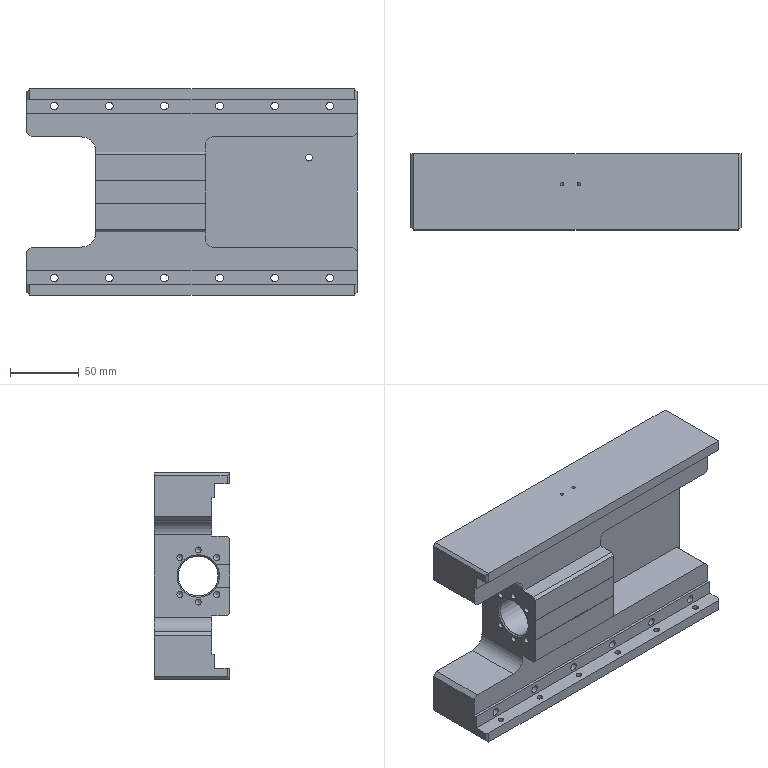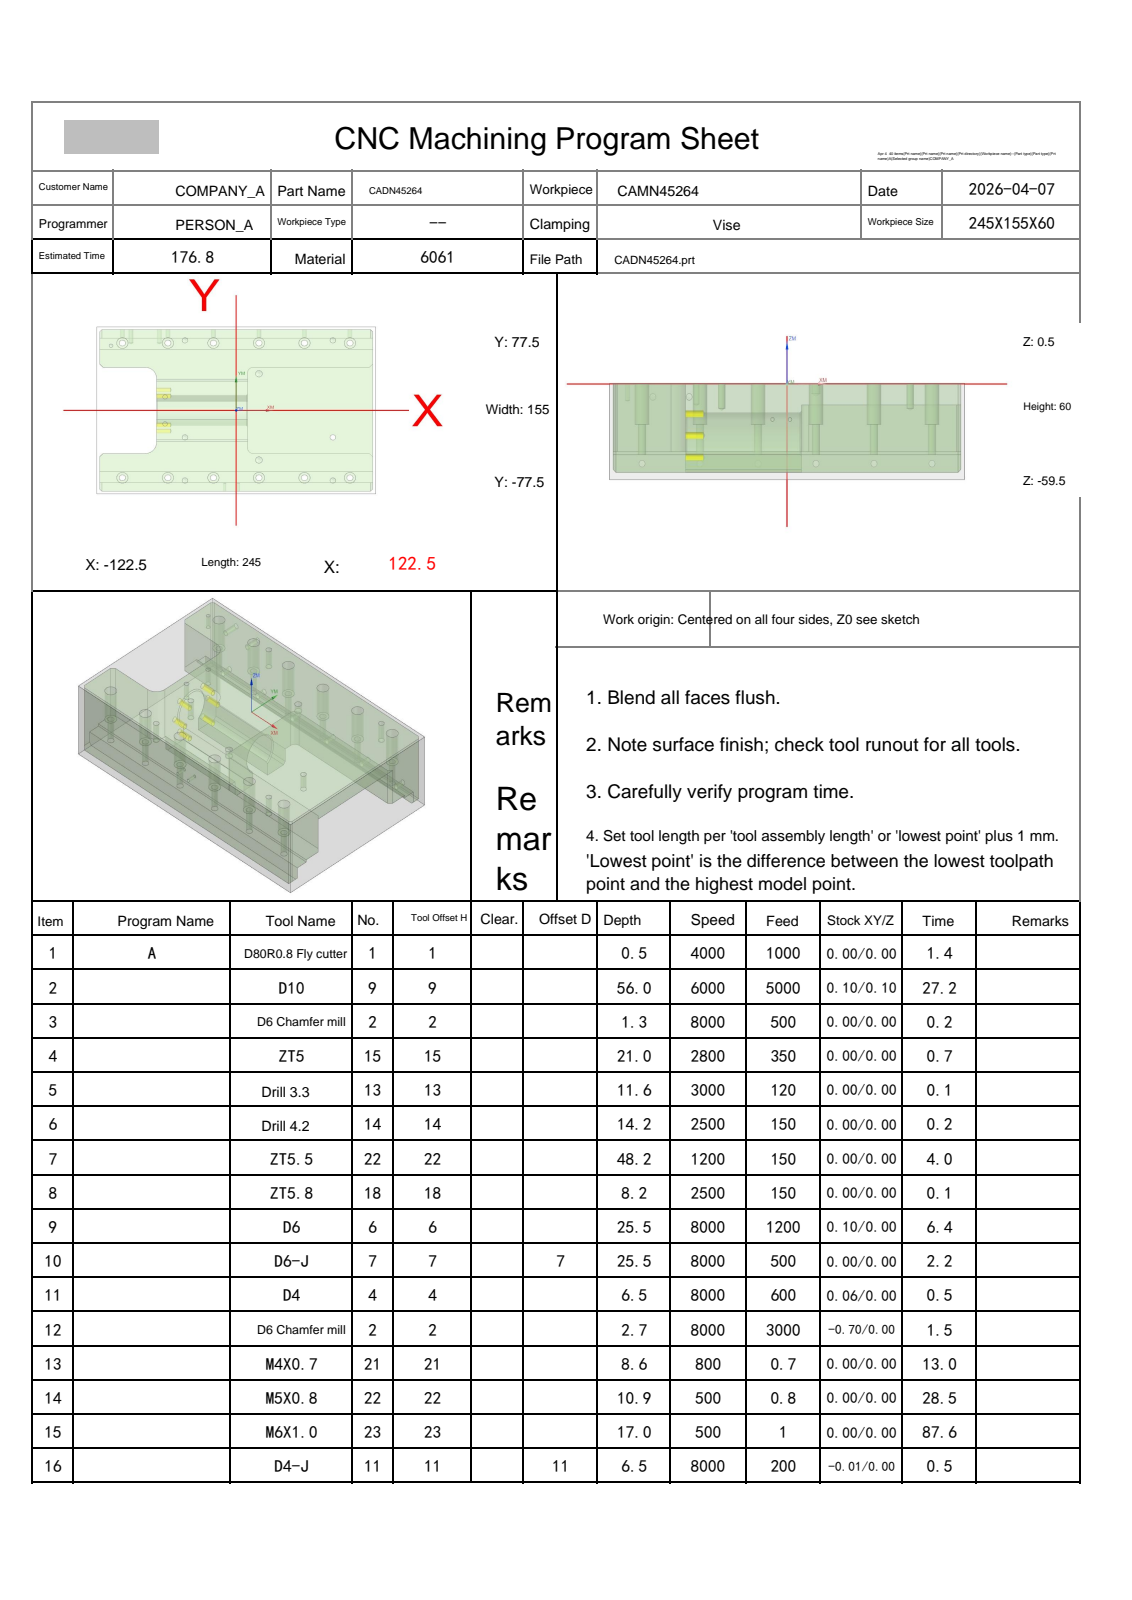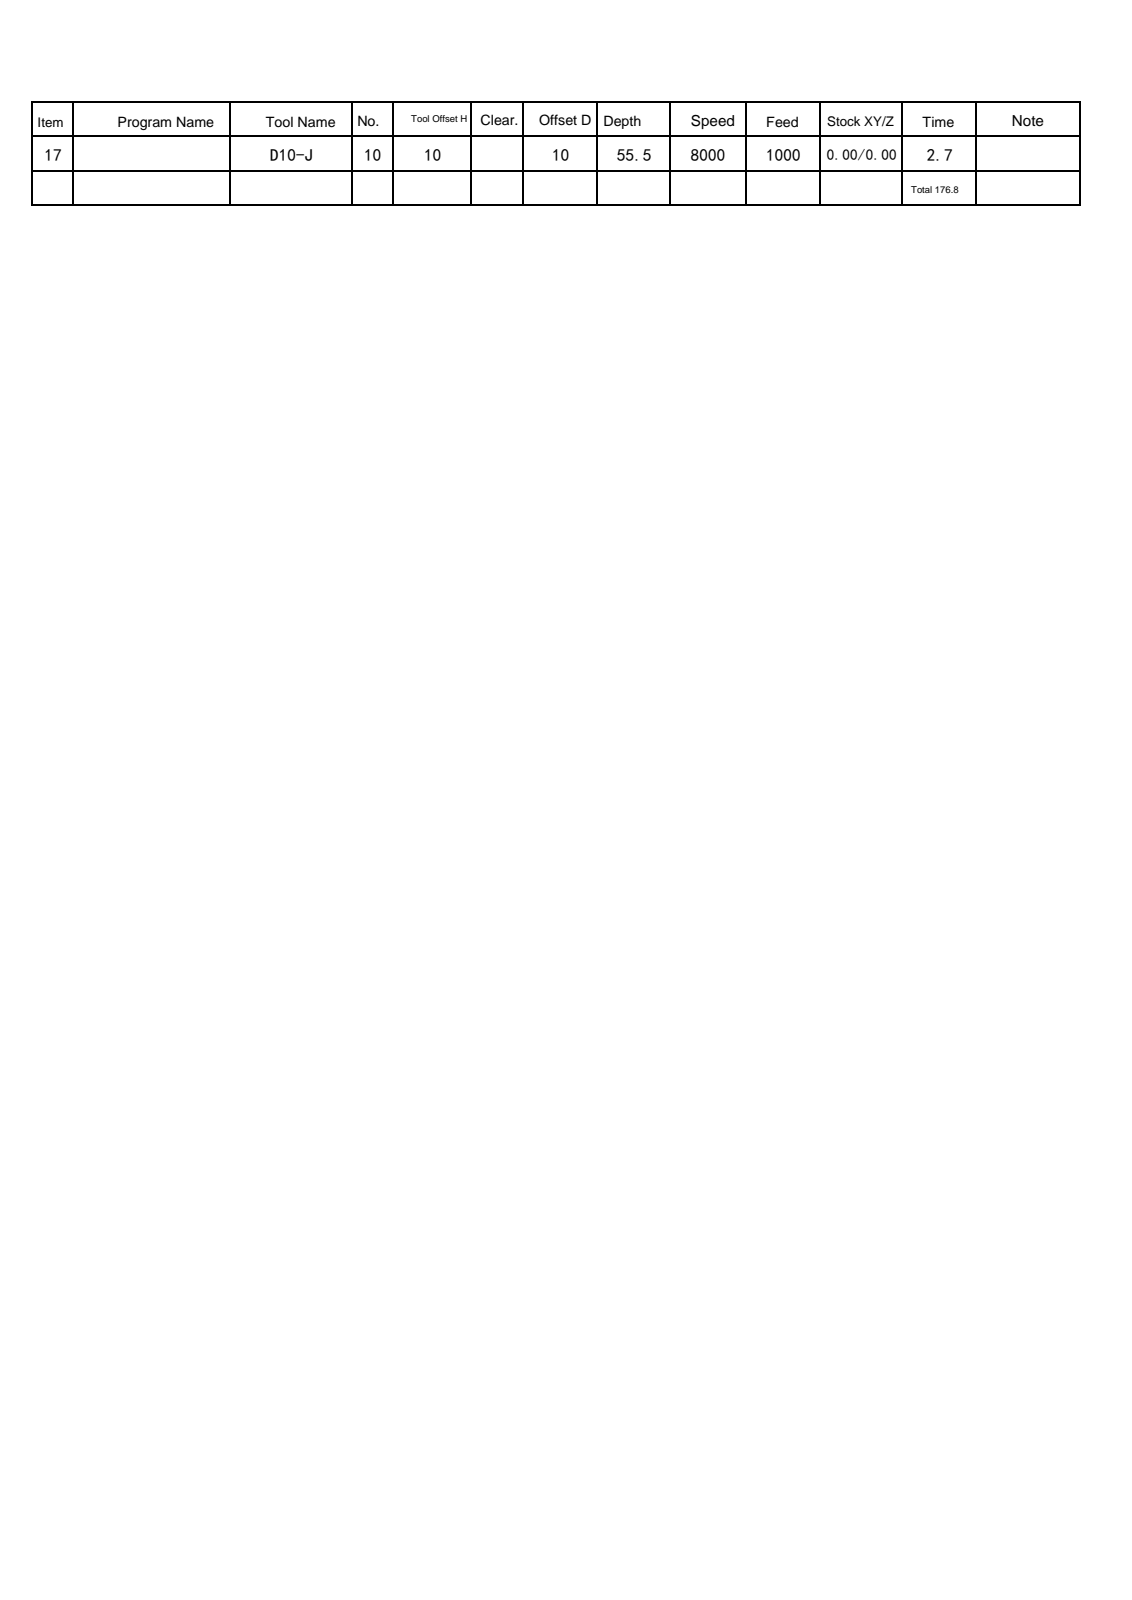NC program | NX | posted by the shop | part box 240 x 55 x 150 mm
Lines 10566 to 12612 of 12612, first 1141 of 2047 lines:
N3 T02 M06
(D6 Chamfer mill  D=6. R=0. H=02 ce=0.00 di=0.10)
G00 G90 G54 X85. Y-25. M03 S8000
G43 H02 Z20.
M08
G98 G81 X85. Y-25. Z-.8 R1. F500.
X100. Y-62.5
X85. Y-65.
X60. Y-62.5
X20.
Y-46.
X-20. Y-62.5
X-45. Y-65.
X-60. Y-62.5
X-100.
X-45. Y-25.
X-62.5 Y-12.5
Y12.5
X-110. Y60.
X-100. Y62.5
X-60.
X-45. Y65.
X-20. Y62.5
X20.
Y34.
X60. Y62.5
X85. Y65.
X100. Y62.5
G80
G00 Z20.
G91 G28 Z0.0
M05
M09
G91 G28 Z0.0
M01
N4 T15 M06
(ZT5 D=5. DR_a=118 H=15)
G00 G90 G54 X85. Y-25. M03 S2800
G43 H15 Z20.
M08
G98 G83 X85. Y-25. Z-20.502 R1. F350. Q3.
G80
G00 Z20.
G00 G90 X85. Y65. M03 S2500
Z20.
G98 G83 X85. Y65. Z-16.502 R1. F150. Q3.
X-45.
Y-25.
Y-65.
X85.
G80
G00 Z20.
G91 G28 Z0.0
M05
M09
G91 G28 Z0.0
M01
N5 T13 M06
(Drill 3.3 D=3.3 DR_a=118 H=13)
G00 G90 G54 X-110. Y60. M03 S3000
G43 H13 Z20.
M08
G98 G83 X-110. Y60. Z-11.091 R1. F120. Q2.
G80
G00 Z20.
G91 G28 Z0.0
M05
M09
G91 G28 Z0.0
M01
N6 T14 M06
(Drill 4.2 D=4.2 DR_a=118 H=14)
G00 G90 G54 X-62.5 Y-12.5 M03 S2500
G43 H14 Z20.
M08
G98 G83 X-62.5 Y-12.5 Z-13.662 R1. F150. Q3.
Y12.5
G80
G00 Z20.
G91 G28 Z0.0
M05
M09
G91 G28 Z0.0
M01
N7 T22 M06
(ZT5.5 D=5.5 DR_a=118 H=22)
G00 G90 G54 X-100. Y-62.5 M03 S1200
G43 H22 Z20.
M08
G98 G83 X-100. Y-62.5 Z-47.652 R1. F150. Q2.
X-60.
X-20.
X20.
X60.
X100.
Y62.5
X60.
X20.
X-20.
X-60.
X-100.
G80
G00 Z20.
G91 G28 Z0.0
M05
M09
G91 G28 Z0.0
M01
N8 T18 M06
(ZT5.8 D=5.8 DR_a=118 H=18)
G00 G90 G54 X20. Y-46. M03 S2500
G43 H18 Z20.
M08
G98 G83 X20. Y-46. Z-7.703 R1. F150. Q2.
Y34.
G80
G00 Z20.
G91 G28 Z0.0
M05
M09
G91 G28 Z0.0
M01
N9 T06 M06
(D6  D=6. R=0. H=06 ce=0.10 di=0.00)
G00 G90 G54 X-100. Y-62.5 M03 S8000
G43 H06 Z20.
M08
Z.5
G03 X-99.05 Y-63.45 I.95 J0.0 F1200.
X-98.1 Y-62.5 I0.0 J.95
X-98.1 Y-62.5 Z0.0 I-1.9 J0.0
X-98.1 Y-62.5 Z-.5 I-1.9 J0.0
X-98.1 Y-62.5 Z-1. I-1.9 J0.0
X-98.1 Y-62.5 Z-1.5 I-1.9 J0.0
X-98.1 Y-62.5 Z-2. I-1.9 J0.0
X-98.1 Y-62.5 Z-2.5 I-1.9 J0.0
X-98.1 Y-62.5 Z-3. I-1.9 J0.0
X-98.1 Y-62.5 Z-3.5 I-1.9 J0.0
X-98.1 Y-62.5 Z-4. I-1.9 J0.0
X-98.1 Y-62.5 Z-4.5 I-1.9 J0.0
X-98.1 Y-62.5 Z-5. I-1.9 J0.0
X-98.1 Y-62.5 Z-5.5 I-1.9 J0.0
X-98.1 Y-62.5 Z-6. I-1.9 J0.0
X-98.1 Y-62.5 Z-6.5 I-1.9 J0.0
X-98.1 Y-62.5 Z-7. I-1.9 J0.0
X-98.1 Y-62.5 Z-7.5 I-1.9 J0.0
X-98.1 Y-62.5 Z-8. I-1.9 J0.0
X-98.1 Y-62.5 Z-8.5 I-1.9 J0.0
X-98.1 Y-62.5 Z-9. I-1.9 J0.0
X-98.1 Y-62.5 Z-9.5 I-1.9 J0.0
X-98.1 Y-62.5 Z-10. I-1.9 J0.0
X-98.1 Y-62.5 Z-10.5 I-1.9 J0.0
X-98.1 Y-62.5 Z-11. I-1.9 J0.0
X-98.1 Y-62.5 Z-11.5 I-1.9 J0.0
X-98.1 Y-62.5 Z-12. I-1.9 J0.0
X-98.1 Y-62.5 Z-12.5 I-1.9 J0.0
X-98.1 Y-62.5 Z-13. I-1.9 J0.0
X-98.1 Y-62.5 Z-13.5 I-1.9 J0.0
X-98.1 Y-62.5 Z-14. I-1.9 J0.0
X-98.1 Y-62.5 Z-14.5 I-1.9 J0.0
X-98.1 Y-62.5 Z-15. I-1.9 J0.0
X-98.1 Y-62.5 Z-15.5 I-1.9 J0.0
X-98.1 Y-62.5 Z-16. I-1.9 J0.0
X-98.1 Y-62.5 Z-16.5 I-1.9 J0.0
X-98.1 Y-62.5 Z-17. I-1.9 J0.0
X-98.1 Y-62.5 Z-17.5 I-1.9 J0.0
X-98.1 Y-62.5 Z-18. I-1.9 J0.0
X-98.1 Y-62.5 Z-18.5 I-1.9 J0.0
X-98.1 Y-62.5 Z-19. I-1.9 J0.0
X-98.1 Y-62.5 Z-19.5 I-1.9 J0.0
X-98.1 Y-62.5 Z-20. I-1.9 J0.0
X-98.1 Y-62.5 Z-20.5 I-1.9 J0.0
X-98.1 Y-62.5 Z-21. I-1.9 J0.0
X-98.1 Y-62.5 Z-21.5 I-1.9 J0.0
X-98.1 Y-62.5 Z-22. I-1.9 J0.0
X-98.1 Y-62.5 Z-22.5 I-1.9 J0.0
X-98.1 Y-62.5 Z-23. I-1.9 J0.0
X-98.1 Y-62.5 Z-23.5 I-1.9 J0.0
X-98.1 Y-62.5 Z-24. I-1.9 J0.0
X-98.1 Y-62.5 Z-24.5 I-1.9 J0.0
X-98.1 Y-62.5 Z-25. I-1.9 J0.0
X-100. Y-60.6 I-1.9 J0.0
X-101.9 Y-62.5 I0.0 J-1.9
X-100. Y-64.4 I1.9 J0.0
X-98.1 Y-62.5 I0.0 J1.9
X-99.05 Y-61.55 I-.95 J0.0
X-100. Y-62.5 I0.0 J-.95
G00 Z20.
X-60.
Z.5
G03 X-59.05 Y-63.45 I.95 J0.0
X-58.1 Y-62.5 I0.0 J.95
X-58.1 Y-62.5 Z0.0 I-1.9 J0.0
X-58.1 Y-62.5 Z-.5 I-1.9 J0.0
X-58.1 Y-62.5 Z-1. I-1.9 J0.0
X-58.1 Y-62.5 Z-1.5 I-1.9 J0.0
X-58.1 Y-62.5 Z-2. I-1.9 J0.0
X-58.1 Y-62.5 Z-2.5 I-1.9 J0.0
X-58.1 Y-62.5 Z-3. I-1.9 J0.0
X-58.1 Y-62.5 Z-3.5 I-1.9 J0.0
X-58.1 Y-62.5 Z-4. I-1.9 J0.0
X-58.1 Y-62.5 Z-4.5 I-1.9 J0.0
X-58.1 Y-62.5 Z-5. I-1.9 J0.0
X-58.1 Y-62.5 Z-5.5 I-1.9 J0.0
X-58.1 Y-62.5 Z-6. I-1.9 J0.0
X-58.1 Y-62.5 Z-6.5 I-1.9 J0.0
X-58.1 Y-62.5 Z-7. I-1.9 J0.0
X-58.1 Y-62.5 Z-7.5 I-1.9 J0.0
X-58.1 Y-62.5 Z-8. I-1.9 J0.0
X-58.1 Y-62.5 Z-8.5 I-1.9 J0.0
X-58.1 Y-62.5 Z-9. I-1.9 J0.0
X-58.1 Y-62.5 Z-9.5 I-1.9 J0.0
X-58.1 Y-62.5 Z-10. I-1.9 J0.0
X-58.1 Y-62.5 Z-10.5 I-1.9 J0.0
X-58.1 Y-62.5 Z-11. I-1.9 J0.0
X-58.1 Y-62.5 Z-11.5 I-1.9 J0.0
X-58.1 Y-62.5 Z-12. I-1.9 J0.0
X-58.1 Y-62.5 Z-12.5 I-1.9 J0.0
X-58.1 Y-62.5 Z-13. I-1.9 J0.0
X-58.1 Y-62.5 Z-13.5 I-1.9 J0.0
X-58.1 Y-62.5 Z-14. I-1.9 J0.0
X-58.1 Y-62.5 Z-14.5 I-1.9 J0.0
X-58.1 Y-62.5 Z-15. I-1.9 J0.0
X-58.1 Y-62.5 Z-15.5 I-1.9 J0.0
X-58.1 Y-62.5 Z-16. I-1.9 J0.0
X-58.1 Y-62.5 Z-16.5 I-1.9 J0.0
X-58.1 Y-62.5 Z-17. I-1.9 J0.0
X-58.1 Y-62.5 Z-17.5 I-1.9 J0.0
X-58.1 Y-62.5 Z-18. I-1.9 J0.0
X-58.1 Y-62.5 Z-18.5 I-1.9 J0.0
X-58.1 Y-62.5 Z-19. I-1.9 J0.0
X-58.1 Y-62.5 Z-19.5 I-1.9 J0.0
X-58.1 Y-62.5 Z-20. I-1.9 J0.0
X-58.1 Y-62.5 Z-20.5 I-1.9 J0.0
X-58.1 Y-62.5 Z-21. I-1.9 J0.0
X-58.1 Y-62.5 Z-21.5 I-1.9 J0.0
X-58.1 Y-62.5 Z-22. I-1.9 J0.0
X-58.1 Y-62.5 Z-22.5 I-1.9 J0.0
X-58.1 Y-62.5 Z-23. I-1.9 J0.0
X-58.1 Y-62.5 Z-23.5 I-1.9 J0.0
X-58.1 Y-62.5 Z-24. I-1.9 J0.0
X-58.1 Y-62.5 Z-24.5 I-1.9 J0.0
X-58.1 Y-62.5 Z-25. I-1.9 J0.0
X-60. Y-60.6 I-1.9 J0.0
X-61.9 Y-62.5 I0.0 J-1.9
X-60. Y-64.4 I1.9 J0.0
X-58.1 Y-62.5 I0.0 J1.9
X-59.05 Y-61.55 I-.95 J0.0
X-60. Y-62.5 I0.0 J-.95
G00 Z20.
X-20.
Z.5
G03 X-19.05 Y-63.45 I.95 J0.0
X-18.1 Y-62.5 I0.0 J.95
X-18.1 Y-62.5 Z0.0 I-1.9 J0.0
X-18.1 Y-62.5 Z-.5 I-1.9 J0.0
X-18.1 Y-62.5 Z-1. I-1.9 J0.0
X-18.1 Y-62.5 Z-1.5 I-1.9 J0.0
X-18.1 Y-62.5 Z-2. I-1.9 J0.0
X-18.1 Y-62.5 Z-2.5 I-1.9 J0.0
X-18.1 Y-62.5 Z-3. I-1.9 J0.0
X-18.1 Y-62.5 Z-3.5 I-1.9 J0.0
X-18.1 Y-62.5 Z-4. I-1.9 J0.0
X-18.1 Y-62.5 Z-4.5 I-1.9 J0.0
X-18.1 Y-62.5 Z-5. I-1.9 J0.0
X-18.1 Y-62.5 Z-5.5 I-1.9 J0.0
X-18.1 Y-62.5 Z-6. I-1.9 J0.0
X-18.1 Y-62.5 Z-6.5 I-1.9 J0.0
X-18.1 Y-62.5 Z-7. I-1.9 J0.0
X-18.1 Y-62.5 Z-7.5 I-1.9 J0.0
X-18.1 Y-62.5 Z-8. I-1.9 J0.0
X-18.1 Y-62.5 Z-8.5 I-1.9 J0.0
X-18.1 Y-62.5 Z-9. I-1.9 J0.0
X-18.1 Y-62.5 Z-9.5 I-1.9 J0.0
X-18.1 Y-62.5 Z-10. I-1.9 J0.0
X-18.1 Y-62.5 Z-10.5 I-1.9 J0.0
X-18.1 Y-62.5 Z-11. I-1.9 J0.0
X-18.1 Y-62.5 Z-11.5 I-1.9 J0.0
X-18.1 Y-62.5 Z-12. I-1.9 J0.0
X-18.1 Y-62.5 Z-12.5 I-1.9 J0.0
X-18.1 Y-62.5 Z-13. I-1.9 J0.0
X-18.1 Y-62.5 Z-13.5 I-1.9 J0.0
X-18.1 Y-62.5 Z-14. I-1.9 J0.0
X-18.1 Y-62.5 Z-14.5 I-1.9 J0.0
X-18.1 Y-62.5 Z-15. I-1.9 J0.0
X-18.1 Y-62.5 Z-15.5 I-1.9 J0.0
X-18.1 Y-62.5 Z-16. I-1.9 J0.0
X-18.1 Y-62.5 Z-16.5 I-1.9 J0.0
X-18.1 Y-62.5 Z-17. I-1.9 J0.0
X-18.1 Y-62.5 Z-17.5 I-1.9 J0.0
X-18.1 Y-62.5 Z-18. I-1.9 J0.0
X-18.1 Y-62.5 Z-18.5 I-1.9 J0.0
X-18.1 Y-62.5 Z-19. I-1.9 J0.0
X-18.1 Y-62.5 Z-19.5 I-1.9 J0.0
X-18.1 Y-62.5 Z-20. I-1.9 J0.0
X-18.1 Y-62.5 Z-20.5 I-1.9 J0.0
X-18.1 Y-62.5 Z-21. I-1.9 J0.0
X-18.1 Y-62.5 Z-21.5 I-1.9 J0.0
X-18.1 Y-62.5 Z-22. I-1.9 J0.0
X-18.1 Y-62.5 Z-22.5 I-1.9 J0.0
X-18.1 Y-62.5 Z-23. I-1.9 J0.0
X-18.1 Y-62.5 Z-23.5 I-1.9 J0.0
X-18.1 Y-62.5 Z-24. I-1.9 J0.0
X-18.1 Y-62.5 Z-24.5 I-1.9 J0.0
X-18.1 Y-62.5 Z-25. I-1.9 J0.0
X-20. Y-60.6 I-1.9 J0.0
X-21.9 Y-62.5 I0.0 J-1.9
X-20. Y-64.4 I1.9 J0.0
X-18.1 Y-62.5 I0.0 J1.9
X-19.05 Y-61.55 I-.95 J0.0
X-20. Y-62.5 I0.0 J-.95
G00 Z20.
X20.
Z.5
G03 X20.95 Y-63.45 I.95 J0.0
X21.9 Y-62.5 I0.0 J.95
X21.9 Y-62.5 Z0.0 I-1.9 J0.0
X21.9 Y-62.5 Z-.5 I-1.9 J0.0
X21.9 Y-62.5 Z-1. I-1.9 J0.0
X21.9 Y-62.5 Z-1.5 I-1.9 J0.0
X21.9 Y-62.5 Z-2. I-1.9 J0.0
X21.9 Y-62.5 Z-2.5 I-1.9 J0.0
X21.9 Y-62.5 Z-3. I-1.9 J0.0
X21.9 Y-62.5 Z-3.5 I-1.9 J0.0
X21.9 Y-62.5 Z-4. I-1.9 J0.0
X21.9 Y-62.5 Z-4.5 I-1.9 J0.0
X21.9 Y-62.5 Z-5. I-1.9 J0.0
X21.9 Y-62.5 Z-5.5 I-1.9 J0.0
X21.9 Y-62.5 Z-6. I-1.9 J0.0
X21.9 Y-62.5 Z-6.5 I-1.9 J0.0
X21.9 Y-62.5 Z-7. I-1.9 J0.0
X21.9 Y-62.5 Z-7.5 I-1.9 J0.0
X21.9 Y-62.5 Z-8. I-1.9 J0.0
X21.9 Y-62.5 Z-8.5 I-1.9 J0.0
X21.9 Y-62.5 Z-9. I-1.9 J0.0
X21.9 Y-62.5 Z-9.5 I-1.9 J0.0
X21.9 Y-62.5 Z-10. I-1.9 J0.0
X21.9 Y-62.5 Z-10.5 I-1.9 J0.0
X21.9 Y-62.5 Z-11. I-1.9 J0.0
X21.9 Y-62.5 Z-11.5 I-1.9 J0.0
X21.9 Y-62.5 Z-12. I-1.9 J0.0
X21.9 Y-62.5 Z-12.5 I-1.9 J0.0
X21.9 Y-62.5 Z-13. I-1.9 J0.0
X21.9 Y-62.5 Z-13.5 I-1.9 J0.0
X21.9 Y-62.5 Z-14. I-1.9 J0.0
X21.9 Y-62.5 Z-14.5 I-1.9 J0.0
X21.9 Y-62.5 Z-15. I-1.9 J0.0
X21.9 Y-62.5 Z-15.5 I-1.9 J0.0
X21.9 Y-62.5 Z-16. I-1.9 J0.0
X21.9 Y-62.5 Z-16.5 I-1.9 J0.0
X21.9 Y-62.5 Z-17. I-1.9 J0.0
X21.9 Y-62.5 Z-17.5 I-1.9 J0.0
X21.9 Y-62.5 Z-18. I-1.9 J0.0
X21.9 Y-62.5 Z-18.5 I-1.9 J0.0
X21.9 Y-62.5 Z-19. I-1.9 J0.0
X21.9 Y-62.5 Z-19.5 I-1.9 J0.0
X21.9 Y-62.5 Z-20. I-1.9 J0.0
X21.9 Y-62.5 Z-20.5 I-1.9 J0.0
X21.9 Y-62.5 Z-21. I-1.9 J0.0
X21.9 Y-62.5 Z-21.5 I-1.9 J0.0
X21.9 Y-62.5 Z-22. I-1.9 J0.0
X21.9 Y-62.5 Z-22.5 I-1.9 J0.0
X21.9 Y-62.5 Z-23. I-1.9 J0.0
X21.9 Y-62.5 Z-23.5 I-1.9 J0.0
X21.9 Y-62.5 Z-24. I-1.9 J0.0
X21.9 Y-62.5 Z-24.5 I-1.9 J0.0
X21.9 Y-62.5 Z-25. I-1.9 J0.0
X20. Y-60.6 I-1.9 J0.0
X18.1 Y-62.5 I0.0 J-1.9
X20. Y-64.4 I1.9 J0.0
X21.9 Y-62.5 I0.0 J1.9
X20.95 Y-61.55 I-.95 J0.0
X20. Y-62.5 I0.0 J-.95
G00 Z20.
X60.
Z.5
G03 X60.95 Y-63.45 I.95 J0.0
X61.9 Y-62.5 I0.0 J.95
X61.9 Y-62.5 Z0.0 I-1.9 J0.0
X61.9 Y-62.5 Z-.5 I-1.9 J0.0
X61.9 Y-62.5 Z-1. I-1.9 J0.0
X61.9 Y-62.5 Z-1.5 I-1.9 J0.0
X61.9 Y-62.5 Z-2. I-1.9 J0.0
X61.9 Y-62.5 Z-2.5 I-1.9 J0.0
X61.9 Y-62.5 Z-3. I-1.9 J0.0
X61.9 Y-62.5 Z-3.5 I-1.9 J0.0
X61.9 Y-62.5 Z-4. I-1.9 J0.0
X61.9 Y-62.5 Z-4.5 I-1.9 J0.0
X61.9 Y-62.5 Z-5. I-1.9 J0.0
X61.9 Y-62.5 Z-5.5 I-1.9 J0.0
X61.9 Y-62.5 Z-6. I-1.9 J0.0
X61.9 Y-62.5 Z-6.5 I-1.9 J0.0
X61.9 Y-62.5 Z-7. I-1.9 J0.0
X61.9 Y-62.5 Z-7.5 I-1.9 J0.0
X61.9 Y-62.5 Z-8. I-1.9 J0.0
X61.9 Y-62.5 Z-8.5 I-1.9 J0.0
X61.9 Y-62.5 Z-9. I-1.9 J0.0
X61.9 Y-62.5 Z-9.5 I-1.9 J0.0
X61.9 Y-62.5 Z-10. I-1.9 J0.0
X61.9 Y-62.5 Z-10.5 I-1.9 J0.0
X61.9 Y-62.5 Z-11. I-1.9 J0.0
X61.9 Y-62.5 Z-11.5 I-1.9 J0.0
X61.9 Y-62.5 Z-12. I-1.9 J0.0
X61.9 Y-62.5 Z-12.5 I-1.9 J0.0
X61.9 Y-62.5 Z-13. I-1.9 J0.0
X61.9 Y-62.5 Z-13.5 I-1.9 J0.0
X61.9 Y-62.5 Z-14. I-1.9 J0.0
X61.9 Y-62.5 Z-14.5 I-1.9 J0.0
X61.9 Y-62.5 Z-15. I-1.9 J0.0
X61.9 Y-62.5 Z-15.5 I-1.9 J0.0
X61.9 Y-62.5 Z-16. I-1.9 J0.0
X61.9 Y-62.5 Z-16.5 I-1.9 J0.0
X61.9 Y-62.5 Z-17. I-1.9 J0.0
X61.9 Y-62.5 Z-17.5 I-1.9 J0.0
X61.9 Y-62.5 Z-18. I-1.9 J0.0
X61.9 Y-62.5 Z-18.5 I-1.9 J0.0
X61.9 Y-62.5 Z-19. I-1.9 J0.0
X61.9 Y-62.5 Z-19.5 I-1.9 J0.0
X61.9 Y-62.5 Z-20. I-1.9 J0.0
X61.9 Y-62.5 Z-20.5 I-1.9 J0.0
X61.9 Y-62.5 Z-21. I-1.9 J0.0
X61.9 Y-62.5 Z-21.5 I-1.9 J0.0
X61.9 Y-62.5 Z-22. I-1.9 J0.0
X61.9 Y-62.5 Z-22.5 I-1.9 J0.0
X61.9 Y-62.5 Z-23. I-1.9 J0.0
X61.9 Y-62.5 Z-23.5 I-1.9 J0.0
X61.9 Y-62.5 Z-24. I-1.9 J0.0
X61.9 Y-62.5 Z-24.5 I-1.9 J0.0
X61.9 Y-62.5 Z-25. I-1.9 J0.0
X60. Y-60.6 I-1.9 J0.0
X58.1 Y-62.5 I0.0 J-1.9
X60. Y-64.4 I1.9 J0.0
X61.9 Y-62.5 I0.0 J1.9
X60.95 Y-61.55 I-.95 J0.0
X60. Y-62.5 I0.0 J-.95
G00 Z20.
X100.
Z.5
G03 X100.95 Y-63.45 I.95 J0.0
X101.9 Y-62.5 I0.0 J.95
X101.9 Y-62.5 Z0.0 I-1.9 J0.0
X101.9 Y-62.5 Z-.5 I-1.9 J0.0
X101.9 Y-62.5 Z-1. I-1.9 J0.0
X101.9 Y-62.5 Z-1.5 I-1.9 J0.0
X101.9 Y-62.5 Z-2. I-1.9 J0.0
X101.9 Y-62.5 Z-2.5 I-1.9 J0.0
X101.9 Y-62.5 Z-3. I-1.9 J0.0
X101.9 Y-62.5 Z-3.5 I-1.9 J0.0
X101.9 Y-62.5 Z-4. I-1.9 J0.0
X101.9 Y-62.5 Z-4.5 I-1.9 J0.0
X101.9 Y-62.5 Z-5. I-1.9 J0.0
X101.9 Y-62.5 Z-5.5 I-1.9 J0.0
X101.9 Y-62.5 Z-6. I-1.9 J0.0
X101.9 Y-62.5 Z-6.5 I-1.9 J0.0
X101.9 Y-62.5 Z-7. I-1.9 J0.0
X101.9 Y-62.5 Z-7.5 I-1.9 J0.0
X101.9 Y-62.5 Z-8. I-1.9 J0.0
X101.9 Y-62.5 Z-8.5 I-1.9 J0.0
X101.9 Y-62.5 Z-9. I-1.9 J0.0
X101.9 Y-62.5 Z-9.5 I-1.9 J0.0
X101.9 Y-62.5 Z-10. I-1.9 J0.0
X101.9 Y-62.5 Z-10.5 I-1.9 J0.0
X101.9 Y-62.5 Z-11. I-1.9 J0.0
X101.9 Y-62.5 Z-11.5 I-1.9 J0.0
X101.9 Y-62.5 Z-12. I-1.9 J0.0
X101.9 Y-62.5 Z-12.5 I-1.9 J0.0
X101.9 Y-62.5 Z-13. I-1.9 J0.0
X101.9 Y-62.5 Z-13.5 I-1.9 J0.0
X101.9 Y-62.5 Z-14. I-1.9 J0.0
X101.9 Y-62.5 Z-14.5 I-1.9 J0.0
X101.9 Y-62.5 Z-15. I-1.9 J0.0
X101.9 Y-62.5 Z-15.5 I-1.9 J0.0
X101.9 Y-62.5 Z-16. I-1.9 J0.0
X101.9 Y-62.5 Z-16.5 I-1.9 J0.0
X101.9 Y-62.5 Z-17. I-1.9 J0.0
X101.9 Y-62.5 Z-17.5 I-1.9 J0.0
X101.9 Y-62.5 Z-18. I-1.9 J0.0
X101.9 Y-62.5 Z-18.5 I-1.9 J0.0
X101.9 Y-62.5 Z-19. I-1.9 J0.0
X101.9 Y-62.5 Z-19.5 I-1.9 J0.0
X101.9 Y-62.5 Z-20. I-1.9 J0.0
X101.9 Y-62.5 Z-20.5 I-1.9 J0.0
X101.9 Y-62.5 Z-21. I-1.9 J0.0
X101.9 Y-62.5 Z-21.5 I-1.9 J0.0
X101.9 Y-62.5 Z-22. I-1.9 J0.0
X101.9 Y-62.5 Z-22.5 I-1.9 J0.0
X101.9 Y-62.5 Z-23. I-1.9 J0.0
X101.9 Y-62.5 Z-23.5 I-1.9 J0.0
X101.9 Y-62.5 Z-24. I-1.9 J0.0
X101.9 Y-62.5 Z-24.5 I-1.9 J0.0
X101.9 Y-62.5 Z-25. I-1.9 J0.0
X100. Y-60.6 I-1.9 J0.0
X98.1 Y-62.5 I0.0 J-1.9
X100. Y-64.4 I1.9 J0.0
X101.9 Y-62.5 I0.0 J1.9
X100.95 Y-61.55 I-.95 J0.0
X100. Y-62.5 I0.0 J-.95
G00 Z20.
Y62.5
Z.5
G03 X100.95 Y61.55 I.95 J0.0
X101.9 Y62.5 I0.0 J.95
X101.9 Y62.5 Z0.0 I-1.9 J0.0
X101.9 Y62.5 Z-.5 I-1.9 J0.0
X101.9 Y62.5 Z-1. I-1.9 J0.0
X101.9 Y62.5 Z-1.5 I-1.9 J0.0
X101.9 Y62.5 Z-2. I-1.9 J0.0
X101.9 Y62.5 Z-2.5 I-1.9 J0.0
X101.9 Y62.5 Z-3. I-1.9 J0.0
X101.9 Y62.5 Z-3.5 I-1.9 J0.0
X101.9 Y62.5 Z-4. I-1.9 J0.0
X101.9 Y62.5 Z-4.5 I-1.9 J0.0
X101.9 Y62.5 Z-5. I-1.9 J0.0
X101.9 Y62.5 Z-5.5 I-1.9 J0.0
X101.9 Y62.5 Z-6. I-1.9 J0.0
X101.9 Y62.5 Z-6.5 I-1.9 J0.0
X101.9 Y62.5 Z-7. I-1.9 J0.0
X101.9 Y62.5 Z-7.5 I-1.9 J0.0
X101.9 Y62.5 Z-8. I-1.9 J0.0
X101.9 Y62.5 Z-8.5 I-1.9 J0.0
X101.9 Y62.5 Z-9. I-1.9 J0.0
X101.9 Y62.5 Z-9.5 I-1.9 J0.0
X101.9 Y62.5 Z-10. I-1.9 J0.0
X101.9 Y62.5 Z-10.5 I-1.9 J0.0
X101.9 Y62.5 Z-11. I-1.9 J0.0
X101.9 Y62.5 Z-11.5 I-1.9 J0.0
X101.9 Y62.5 Z-12. I-1.9 J0.0
X101.9 Y62.5 Z-12.5 I-1.9 J0.0
X101.9 Y62.5 Z-13. I-1.9 J0.0
X101.9 Y62.5 Z-13.5 I-1.9 J0.0
X101.9 Y62.5 Z-14. I-1.9 J0.0
X101.9 Y62.5 Z-14.5 I-1.9 J0.0
X101.9 Y62.5 Z-15. I-1.9 J0.0
X101.9 Y62.5 Z-15.5 I-1.9 J0.0
X101.9 Y62.5 Z-16. I-1.9 J0.0
X101.9 Y62.5 Z-16.5 I-1.9 J0.0
X101.9 Y62.5 Z-17. I-1.9 J0.0
X101.9 Y62.5 Z-17.5 I-1.9 J0.0
X101.9 Y62.5 Z-18. I-1.9 J0.0
X101.9 Y62.5 Z-18.5 I-1.9 J0.0
X101.9 Y62.5 Z-19. I-1.9 J0.0
X101.9 Y62.5 Z-19.5 I-1.9 J0.0
X101.9 Y62.5 Z-20. I-1.9 J0.0
X101.9 Y62.5 Z-20.5 I-1.9 J0.0
X101.9 Y62.5 Z-21. I-1.9 J0.0
X101.9 Y62.5 Z-21.5 I-1.9 J0.0
X101.9 Y62.5 Z-22. I-1.9 J0.0
X101.9 Y62.5 Z-22.5 I-1.9 J0.0
X101.9 Y62.5 Z-23. I-1.9 J0.0
X101.9 Y62.5 Z-23.5 I-1.9 J0.0
X101.9 Y62.5 Z-24. I-1.9 J0.0
X101.9 Y62.5 Z-24.5 I-1.9 J0.0
X101.9 Y62.5 Z-25. I-1.9 J0.0
X100. Y64.4 I-1.9 J0.0
X98.1 Y62.5 I0.0 J-1.9
X100. Y60.6 I1.9 J0.0
X101.9 Y62.5 I0.0 J1.9
X100.95 Y63.45 I-.95 J0.0
X100. Y62.5 I0.0 J-.95
G00 Z20.
X60.
Z.5
G03 X60.95 Y61.55 I.95 J0.0
X61.9 Y62.5 I0.0 J.95
X61.9 Y62.5 Z0.0 I-1.9 J0.0
X61.9 Y62.5 Z-.5 I-1.9 J0.0
X61.9 Y62.5 Z-1. I-1.9 J0.0
X61.9 Y62.5 Z-1.5 I-1.9 J0.0
X61.9 Y62.5 Z-2. I-1.9 J0.0
X61.9 Y62.5 Z-2.5 I-1.9 J0.0
X61.9 Y62.5 Z-3. I-1.9 J0.0
X61.9 Y62.5 Z-3.5 I-1.9 J0.0
X61.9 Y62.5 Z-4. I-1.9 J0.0
X61.9 Y62.5 Z-4.5 I-1.9 J0.0
X61.9 Y62.5 Z-5. I-1.9 J0.0
X61.9 Y62.5 Z-5.5 I-1.9 J0.0
X61.9 Y62.5 Z-6. I-1.9 J0.0
X61.9 Y62.5 Z-6.5 I-1.9 J0.0
X61.9 Y62.5 Z-7. I-1.9 J0.0
X61.9 Y62.5 Z-7.5 I-1.9 J0.0
X61.9 Y62.5 Z-8. I-1.9 J0.0
X61.9 Y62.5 Z-8.5 I-1.9 J0.0
X61.9 Y62.5 Z-9. I-1.9 J0.0
X61.9 Y62.5 Z-9.5 I-1.9 J0.0
X61.9 Y62.5 Z-10. I-1.9 J0.0
X61.9 Y62.5 Z-10.5 I-1.9 J0.0
X61.9 Y62.5 Z-11. I-1.9 J0.0
X61.9 Y62.5 Z-11.5 I-1.9 J0.0
X61.9 Y62.5 Z-12. I-1.9 J0.0
X61.9 Y62.5 Z-12.5 I-1.9 J0.0
X61.9 Y62.5 Z-13. I-1.9 J0.0
X61.9 Y62.5 Z-13.5 I-1.9 J0.0
X61.9 Y62.5 Z-14. I-1.9 J0.0
X61.9 Y62.5 Z-14.5 I-1.9 J0.0
X61.9 Y62.5 Z-15. I-1.9 J0.0
X61.9 Y62.5 Z-15.5 I-1.9 J0.0
X61.9 Y62.5 Z-16. I-1.9 J0.0
X61.9 Y62.5 Z-16.5 I-1.9 J0.0
X61.9 Y62.5 Z-17. I-1.9 J0.0
X61.9 Y62.5 Z-17.5 I-1.9 J0.0
X61.9 Y62.5 Z-18. I-1.9 J0.0
X61.9 Y62.5 Z-18.5 I-1.9 J0.0
X61.9 Y62.5 Z-19. I-1.9 J0.0
X61.9 Y62.5 Z-19.5 I-1.9 J0.0
X61.9 Y62.5 Z-20. I-1.9 J0.0
X61.9 Y62.5 Z-20.5 I-1.9 J0.0
X61.9 Y62.5 Z-21. I-1.9 J0.0
X61.9 Y62.5 Z-21.5 I-1.9 J0.0
X61.9 Y62.5 Z-22. I-1.9 J0.0
X61.9 Y62.5 Z-22.5 I-1.9 J0.0
X61.9 Y62.5 Z-23. I-1.9 J0.0
X61.9 Y62.5 Z-23.5 I-1.9 J0.0
X61.9 Y62.5 Z-24. I-1.9 J0.0
X61.9 Y62.5 Z-24.5 I-1.9 J0.0
X61.9 Y62.5 Z-25. I-1.9 J0.0
X60. Y64.4 I-1.9 J0.0
X58.1 Y62.5 I0.0 J-1.9
X60. Y60.6 I1.9 J0.0
X61.9 Y62.5 I0.0 J1.9
X60.95 Y63.45 I-.95 J0.0
X60. Y62.5 I0.0 J-.95
G00 Z20.
X20.
Z.5
G03 X20.95 Y61.55 I.95 J0.0
X21.9 Y62.5 I0.0 J.95
X21.9 Y62.5 Z0.0 I-1.9 J0.0
X21.9 Y62.5 Z-.5 I-1.9 J0.0
X21.9 Y62.5 Z-1. I-1.9 J0.0
X21.9 Y62.5 Z-1.5 I-1.9 J0.0
X21.9 Y62.5 Z-2. I-1.9 J0.0
X21.9 Y62.5 Z-2.5 I-1.9 J0.0
X21.9 Y62.5 Z-3. I-1.9 J0.0
X21.9 Y62.5 Z-3.5 I-1.9 J0.0
X21.9 Y62.5 Z-4. I-1.9 J0.0
X21.9 Y62.5 Z-4.5 I-1.9 J0.0
X21.9 Y62.5 Z-5. I-1.9 J0.0
X21.9 Y62.5 Z-5.5 I-1.9 J0.0
X21.9 Y62.5 Z-6. I-1.9 J0.0
X21.9 Y62.5 Z-6.5 I-1.9 J0.0
X21.9 Y62.5 Z-7. I-1.9 J0.0
X21.9 Y62.5 Z-7.5 I-1.9 J0.0
X21.9 Y62.5 Z-8. I-1.9 J0.0
X21.9 Y62.5 Z-8.5 I-1.9 J0.0
X21.9 Y62.5 Z-9. I-1.9 J0.0
X21.9 Y62.5 Z-9.5 I-1.9 J0.0
X21.9 Y62.5 Z-10. I-1.9 J0.0
X21.9 Y62.5 Z-10.5 I-1.9 J0.0
X21.9 Y62.5 Z-11. I-1.9 J0.0
X21.9 Y62.5 Z-11.5 I-1.9 J0.0
X21.9 Y62.5 Z-12. I-1.9 J0.0
X21.9 Y62.5 Z-12.5 I-1.9 J0.0
X21.9 Y62.5 Z-13. I-1.9 J0.0
X21.9 Y62.5 Z-13.5 I-1.9 J0.0
X21.9 Y62.5 Z-14. I-1.9 J0.0
X21.9 Y62.5 Z-14.5 I-1.9 J0.0
X21.9 Y62.5 Z-15. I-1.9 J0.0
X21.9 Y62.5 Z-15.5 I-1.9 J0.0
X21.9 Y62.5 Z-16. I-1.9 J0.0
X21.9 Y62.5 Z-16.5 I-1.9 J0.0
X21.9 Y62.5 Z-17. I-1.9 J0.0
X21.9 Y62.5 Z-17.5 I-1.9 J0.0
X21.9 Y62.5 Z-18. I-1.9 J0.0
X21.9 Y62.5 Z-18.5 I-1.9 J0.0
X21.9 Y62.5 Z-19. I-1.9 J0.0
X21.9 Y62.5 Z-19.5 I-1.9 J0.0
X21.9 Y62.5 Z-20. I-1.9 J0.0
X21.9 Y62.5 Z-20.5 I-1.9 J0.0
X21.9 Y62.5 Z-21. I-1.9 J0.0
X21.9 Y62.5 Z-21.5 I-1.9 J0.0
X21.9 Y62.5 Z-22. I-1.9 J0.0
X21.9 Y62.5 Z-22.5 I-1.9 J0.0
X21.9 Y62.5 Z-23. I-1.9 J0.0
X21.9 Y62.5 Z-23.5 I-1.9 J0.0
X21.9 Y62.5 Z-24. I-1.9 J0.0
X21.9 Y62.5 Z-24.5 I-1.9 J0.0
X21.9 Y62.5 Z-25. I-1.9 J0.0
X20. Y64.4 I-1.9 J0.0
X18.1 Y62.5 I0.0 J-1.9
X20. Y60.6 I1.9 J0.0
X21.9 Y62.5 I0.0 J1.9
X20.95 Y63.45 I-.95 J0.0
X20. Y62.5 I0.0 J-.95
G00 Z20.
X-20.
Z.5
G03 X-19.05 Y61.55 I.95 J0.0
X-18.1 Y62.5 I0.0 J.95
X-18.1 Y62.5 Z0.0 I-1.9 J0.0
X-18.1 Y62.5 Z-.5 I-1.9 J0.0
X-18.1 Y62.5 Z-1. I-1.9 J0.0
X-18.1 Y62.5 Z-1.5 I-1.9 J0.0
X-18.1 Y62.5 Z-2. I-1.9 J0.0
X-18.1 Y62.5 Z-2.5 I-1.9 J0.0
X-18.1 Y62.5 Z-3. I-1.9 J0.0
X-18.1 Y62.5 Z-3.5 I-1.9 J0.0
X-18.1 Y62.5 Z-4. I-1.9 J0.0
X-18.1 Y62.5 Z-4.5 I-1.9 J0.0
X-18.1 Y62.5 Z-5. I-1.9 J0.0
X-18.1 Y62.5 Z-5.5 I-1.9 J0.0
X-18.1 Y62.5 Z-6. I-1.9 J0.0
X-18.1 Y62.5 Z-6.5 I-1.9 J0.0
X-18.1 Y62.5 Z-7. I-1.9 J0.0
X-18.1 Y62.5 Z-7.5 I-1.9 J0.0
X-18.1 Y62.5 Z-8. I-1.9 J0.0
X-18.1 Y62.5 Z-8.5 I-1.9 J0.0
X-18.1 Y62.5 Z-9. I-1.9 J0.0
X-18.1 Y62.5 Z-9.5 I-1.9 J0.0
X-18.1 Y62.5 Z-10. I-1.9 J0.0
X-18.1 Y62.5 Z-10.5 I-1.9 J0.0
X-18.1 Y62.5 Z-11. I-1.9 J0.0
X-18.1 Y62.5 Z-11.5 I-1.9 J0.0
X-18.1 Y62.5 Z-12. I-1.9 J0.0
X-18.1 Y62.5 Z-12.5 I-1.9 J0.0
X-18.1 Y62.5 Z-13. I-1.9 J0.0
X-18.1 Y62.5 Z-13.5 I-1.9 J0.0
X-18.1 Y62.5 Z-14. I-1.9 J0.0
X-18.1 Y62.5 Z-14.5 I-1.9 J0.0
X-18.1 Y62.5 Z-15. I-1.9 J0.0
X-18.1 Y62.5 Z-15.5 I-1.9 J0.0
X-18.1 Y62.5 Z-16. I-1.9 J0.0
X-18.1 Y62.5 Z-16.5 I-1.9 J0.0
X-18.1 Y62.5 Z-17. I-1.9 J0.0
X-18.1 Y62.5 Z-17.5 I-1.9 J0.0
X-18.1 Y62.5 Z-18. I-1.9 J0.0
X-18.1 Y62.5 Z-18.5 I-1.9 J0.0
X-18.1 Y62.5 Z-19. I-1.9 J0.0
X-18.1 Y62.5 Z-19.5 I-1.9 J0.0
X-18.1 Y62.5 Z-20. I-1.9 J0.0
X-18.1 Y62.5 Z-20.5 I-1.9 J0.0
X-18.1 Y62.5 Z-21. I-1.9 J0.0
X-18.1 Y62.5 Z-21.5 I-1.9 J0.0
X-18.1 Y62.5 Z-22. I-1.9 J0.0
X-18.1 Y62.5 Z-22.5 I-1.9 J0.0
X-18.1 Y62.5 Z-23. I-1.9 J0.0
X-18.1 Y62.5 Z-23.5 I-1.9 J0.0
X-18.1 Y62.5 Z-24. I-1.9 J0.0
X-18.1 Y62.5 Z-24.5 I-1.9 J0.0
X-18.1 Y62.5 Z-25. I-1.9 J0.0
X-20. Y64.4 I-1.9 J0.0
X-21.9 Y62.5 I0.0 J-1.9
X-20. Y60.6 I1.9 J0.0
X-18.1 Y62.5 I0.0 J1.9
X-19.05 Y63.45 I-.95 J0.0
X-20. Y62.5 I0.0 J-.95
G00 Z20.
X-60.
Z.5
G03 X-59.05 Y61.55 I.95 J0.0
X-58.1 Y62.5 I0.0 J.95
X-58.1 Y62.5 Z0.0 I-1.9 J0.0
X-58.1 Y62.5 Z-.5 I-1.9 J0.0
X-58.1 Y62.5 Z-1. I-1.9 J0.0
X-58.1 Y62.5 Z-1.5 I-1.9 J0.0
X-58.1 Y62.5 Z-2. I-1.9 J0.0
X-58.1 Y62.5 Z-2.5 I-1.9 J0.0
X-58.1 Y62.5 Z-3. I-1.9 J0.0
X-58.1 Y62.5 Z-3.5 I-1.9 J0.0
X-58.1 Y62.5 Z-4. I-1.9 J0.0
X-58.1 Y62.5 Z-4.5 I-1.9 J0.0
X-58.1 Y62.5 Z-5. I-1.9 J0.0
X-58.1 Y62.5 Z-5.5 I-1.9 J0.0
X-58.1 Y62.5 Z-6. I-1.9 J0.0
X-58.1 Y62.5 Z-6.5 I-1.9 J0.0
X-58.1 Y62.5 Z-7. I-1.9 J0.0
X-58.1 Y62.5 Z-7.5 I-1.9 J0.0
X-58.1 Y62.5 Z-8. I-1.9 J0.0
X-58.1 Y62.5 Z-8.5 I-1.9 J0.0
X-58.1 Y62.5 Z-9. I-1.9 J0.0
X-58.1 Y62.5 Z-9.5 I-1.9 J0.0
X-58.1 Y62.5 Z-10. I-1.9 J0.0
X-58.1 Y62.5 Z-10.5 I-1.9 J0.0
X-58.1 Y62.5 Z-11. I-1.9 J0.0
X-58.1 Y62.5 Z-11.5 I-1.9 J0.0
X-58.1 Y62.5 Z-12. I-1.9 J0.0
X-58.1 Y62.5 Z-12.5 I-1.9 J0.0
X-58.1 Y62.5 Z-13. I-1.9 J0.0
X-58.1 Y62.5 Z-13.5 I-1.9 J0.0
X-58.1 Y62.5 Z-14. I-1.9 J0.0
X-58.1 Y62.5 Z-14.5 I-1.9 J0.0
X-58.1 Y62.5 Z-15. I-1.9 J0.0
X-58.1 Y62.5 Z-15.5 I-1.9 J0.0
X-58.1 Y62.5 Z-16. I-1.9 J0.0
X-58.1 Y62.5 Z-16.5 I-1.9 J0.0
X-58.1 Y62.5 Z-17. I-1.9 J0.0
X-58.1 Y62.5 Z-17.5 I-1.9 J0.0
X-58.1 Y62.5 Z-18. I-1.9 J0.0
X-58.1 Y62.5 Z-18.5 I-1.9 J0.0
X-58.1 Y62.5 Z-19. I-1.9 J0.0
X-58.1 Y62.5 Z-19.5 I-1.9 J0.0
X-58.1 Y62.5 Z-20. I-1.9 J0.0
X-58.1 Y62.5 Z-20.5 I-1.9 J0.0
X-58.1 Y62.5 Z-21. I-1.9 J0.0
X-58.1 Y62.5 Z-21.5 I-1.9 J0.0
X-58.1 Y62.5 Z-22. I-1.9 J0.0
X-58.1 Y62.5 Z-22.5 I-1.9 J0.0
X-58.1 Y62.5 Z-23. I-1.9 J0.0
X-58.1 Y62.5 Z-23.5 I-1.9 J0.0
X-58.1 Y62.5 Z-24. I-1.9 J0.0
X-58.1 Y62.5 Z-24.5 I-1.9 J0.0
X-58.1 Y62.5 Z-25. I-1.9 J0.0
X-60. Y64.4 I-1.9 J0.0
X-61.9 Y62.5 I0.0 J-1.9
X-60. Y60.6 I1.9 J0.0
X-58.1 Y62.5 I0.0 J1.9
X-59.05 Y63.45 I-.95 J0.0
X-60. Y62.5 I0.0 J-.95
G00 Z20.
X-100.
Z.5
G03 X-99.05 Y61.55 I.95 J0.0
X-98.1 Y62.5 I0.0 J.95
X-98.1 Y62.5 Z0.0 I-1.9 J0.0
X-98.1 Y62.5 Z-.5 I-1.9 J0.0
X-98.1 Y62.5 Z-1. I-1.9 J0.0
X-98.1 Y62.5 Z-1.5 I-1.9 J0.0
X-98.1 Y62.5 Z-2. I-1.9 J0.0
X-98.1 Y62.5 Z-2.5 I-1.9 J0.0
X-98.1 Y62.5 Z-3. I-1.9 J0.0
X-98.1 Y62.5 Z-3.5 I-1.9 J0.0
X-98.1 Y62.5 Z-4. I-1.9 J0.0
X-98.1 Y62.5 Z-4.5 I-1.9 J0.0
X-98.1 Y62.5 Z-5. I-1.9 J0.0
X-98.1 Y62.5 Z-5.5 I-1.9 J0.0
X-98.1 Y62.5 Z-6. I-1.9 J0.0
X-98.1 Y62.5 Z-6.5 I-1.9 J0.0
X-98.1 Y62.5 Z-7. I-1.9 J0.0
X-98.1 Y62.5 Z-7.5 I-1.9 J0.0
X-98.1 Y62.5 Z-8. I-1.9 J0.0
X-98.1 Y62.5 Z-8.5 I-1.9 J0.0
X-98.1 Y62.5 Z-9. I-1.9 J0.0
X-98.1 Y62.5 Z-9.5 I-1.9 J0.0
X-98.1 Y62.5 Z-10. I-1.9 J0.0
X-98.1 Y62.5 Z-10.5 I-1.9 J0.0
X-98.1 Y62.5 Z-11. I-1.9 J0.0
X-98.1 Y62.5 Z-11.5 I-1.9 J0.0
X-98.1 Y62.5 Z-12. I-1.9 J0.0
X-98.1 Y62.5 Z-12.5 I-1.9 J0.0
X-98.1 Y62.5 Z-13. I-1.9 J0.0
X-98.1 Y62.5 Z-13.5 I-1.9 J0.0
X-98.1 Y62.5 Z-14. I-1.9 J0.0
X-98.1 Y62.5 Z-14.5 I-1.9 J0.0
X-98.1 Y62.5 Z-15. I-1.9 J0.0
X-98.1 Y62.5 Z-15.5 I-1.9 J0.0
X-98.1 Y62.5 Z-16. I-1.9 J0.0
X-98.1 Y62.5 Z-16.5 I-1.9 J0.0
X-98.1 Y62.5 Z-17. I-1.9 J0.0
X-98.1 Y62.5 Z-17.5 I-1.9 J0.0
X-98.1 Y62.5 Z-18. I-1.9 J0.0
X-98.1 Y62.5 Z-18.5 I-1.9 J0.0
X-98.1 Y62.5 Z-19. I-1.9 J0.0
X-98.1 Y62.5 Z-19.5 I-1.9 J0.0
X-98.1 Y62.5 Z-20. I-1.9 J0.0
X-98.1 Y62.5 Z-20.5 I-1.9 J0.0
X-98.1 Y62.5 Z-21. I-1.9 J0.0
X-98.1 Y62.5 Z-21.5 I-1.9 J0.0
X-98.1 Y62.5 Z-22. I-1.9 J0.0
X-98.1 Y62.5 Z-22.5 I-1.9 J0.0
X-98.1 Y62.5 Z-23. I-1.9 J0.0
X-98.1 Y62.5 Z-23.5 I-1.9 J0.0
X-98.1 Y62.5 Z-24. I-1.9 J0.0
X-98.1 Y62.5 Z-24.5 I-1.9 J0.0
X-98.1 Y62.5 Z-25. I-1.9 J0.0
X-100. Y64.4 I-1.9 J0.0
X-101.9 Y62.5 I0.0 J-1.9
X-100. Y60.6 I1.9 J0.0
X-98.1 Y62.5 I0.0 J1.9
X-99.05 Y63.45 I-.95 J0.0
X-100. Y62.5 I0.0 J-.95
G00 Z20.
G91 G28 Z0.0
M05
M09
G91 G28 Z0.0
M01
N10 T07 M06
(D6-J  D=6. R=0. H=07 ce=0.00 di=0.00)
G00 G90 G54 X-100. Y-62.5 M03 S8000
G43 H07 Z20.
M08
Z0.0
G41 D07
G01 X-99.96 Y-62.696 F500.
G03 X-98.99 Y-63.49 I.97 J.196
X-98. Y-62.5 I0.0 J.99
X-98. Y-62.5 Z-5. I-2. J0.0
X-98. Y-62.5 Z-10. I-2. J0.0
X-98. Y-62.5 Z-15. I-2. J0.0
X-98. Y-62.5 Z-20. I-2. J0.0
X-98. Y-62.5 Z-25. I-2. J0.0
X-100. Y-60.5 I-2. J0.0
X-102. Y-62.5 I0.0 J-2.
X-100. Y-64.5 I2. J0.0
X-98. Y-62.5 I0.0 J2.
X-98.99 Y-61.51 I-.99 J0.0
X-99.96 Y-62.304 I0.0 J-.99
G01 G40 X-100. Y-62.5
G00 Z20.
X-60.
Z0.0
G41 D07
G01 X-59.96 Y-62.696
G03 X-58.99 Y-63.49 I.97 J.196
X-58. Y-62.5 I0.0 J.99
X-58. Y-62.5 Z-5. I-2. J0.0
X-58. Y-62.5 Z-10. I-2. J0.0
X-58. Y-62.5 Z-15. I-2. J0.0
X-58. Y-62.5 Z-20. I-2. J0.0
X-58. Y-62.5 Z-25. I-2. J0.0
X-60. Y-60.5 I-2. J0.0
X-62. Y-62.5 I0.0 J-2.
X-60. Y-64.5 I2. J0.0
X-58. Y-62.5 I0.0 J2.
X-58.99 Y-61.51 I-.99 J0.0
X-59.96 Y-62.304 I0.0 J-.99
G01 G40 X-60. Y-62.5
G00 Z20.
X-20.
Z0.0
G41 D07
G01 X-19.96 Y-62.696
G03 X-18.99 Y-63.49 I.97 J.196
X-18. Y-62.5 I0.0 J.99
X-18. Y-62.5 Z-5. I-2. J0.0
X-18. Y-62.5 Z-10. I-2. J0.0
X-18. Y-62.5 Z-15. I-2. J0.0
X-18. Y-62.5 Z-20. I-2. J0.0
X-18. Y-62.5 Z-25. I-2. J0.0
X-20. Y-60.5 I-2. J0.0
X-22. Y-62.5 I0.0 J-2.
X-20. Y-64.5 I2. J0.0
X-18. Y-62.5 I0.0 J2.
X-18.99 Y-61.51 I-.99 J0.0
X-19.96 Y-62.304 I0.0 J-.99
G01 G40 X-20. Y-62.5
G00 Z20.
X20.
Z0.0
G41 D07
G01 X20.04 Y-62.696
G03 X21.01 Y-63.49 I.97 J.196
X22. Y-62.5 I0.0 J.99
X22. Y-62.5 Z-5. I-2. J0.0
X22. Y-62.5 Z-10. I-2. J0.0
X22. Y-62.5 Z-15. I-2. J0.0
X22. Y-62.5 Z-20. I-2. J0.0
X22. Y-62.5 Z-25. I-2. J0.0
X20. Y-60.5 I-2. J0.0
X18. Y-62.5 I0.0 J-2.
X20. Y-64.5 I2. J0.0
X22. Y-62.5 I0.0 J2.
X21.01 Y-61.51 I-.99 J0.0
X20.04 Y-62.304 I0.0 J-.99
G01 G40 X20. Y-62.5
G00 Z20.
X60.
Z0.0
G41 D07
G01 X60.04 Y-62.696
G03 X61.01 Y-63.49 I.97 J.196
X62. Y-62.5 I0.0 J.99
X62. Y-62.5 Z-5. I-2. J0.0
X62. Y-62.5 Z-10. I-2. J0.0
X62. Y-62.5 Z-15. I-2. J0.0
X62. Y-62.5 Z-20. I-2. J0.0
X62. Y-62.5 Z-25. I-2. J0.0
X60. Y-60.5 I-2. J0.0
X58. Y-62.5 I0.0 J-2.
X60. Y-64.5 I2. J0.0
X62. Y-62.5 I0.0 J2.
X61.01 Y-61.51 I-.99 J0.0
X60.04 Y-62.304 I0.0 J-.99
G01 G40 X60. Y-62.5
G00 Z20.
X100.
Z0.0
G41 D07
G01 X100.04 Y-62.696
G03 X101.01 Y-63.49 I.97 J.196
X102. Y-62.5 I0.0 J.99
X102. Y-62.5 Z-5. I-2. J0.0
X102. Y-62.5 Z-10. I-2. J0.0
X102. Y-62.5 Z-15. I-2. J0.0
X102. Y-62.5 Z-20. I-2. J0.0
X102. Y-62.5 Z-25. I-2. J0.0
X100. Y-60.5 I-2. J0.0
X98. Y-62.5 I0.0 J-2.
X100. Y-64.5 I2. J0.0
X102. Y-62.5 I0.0 J2.
X101.01 Y-61.51 I-.99 J0.0
X100.04 Y-62.304 I0.0 J-.99
G01 G40 X100. Y-62.5
G00 Z20.
Y62.5
Z0.0
G41 D07
G01 X100.04 Y62.304
G03 X101.01 Y61.51 I.97 J.196
X102. Y62.5 I0.0 J.99
X102. Y62.5 Z-5. I-2. J0.0
X102. Y62.5 Z-10. I-2. J0.0
X102. Y62.5 Z-15. I-2. J0.0
X102. Y62.5 Z-20. I-2. J0.0
X102. Y62.5 Z-25. I-2. J0.0
X100. Y64.5 I-2. J0.0
X98. Y62.5 I0.0 J-2.
X100. Y60.5 I2. J0.0
X102. Y62.5 I0.0 J2.
X101.01 Y63.49 I-.99 J0.0
X100.04 Y62.696 I0.0 J-.99
G01 G40 X100. Y62.5
G00 Z20.
X60.
Z0.0
G41 D07
G01 X60.04 Y62.304
G03 X61.01 Y61.51 I.97 J.196
X62. Y62.5 I0.0 J.99
X62. Y62.5 Z-5. I-2. J0.0
X62. Y62.5 Z-10. I-2. J0.0
X62. Y62.5 Z-15. I-2. J0.0
X62. Y62.5 Z-20. I-2. J0.0
X62. Y62.5 Z-25. I-2. J0.0
X60. Y64.5 I-2. J0.0
X58. Y62.5 I0.0 J-2.
X60. Y60.5 I2. J0.0
X62. Y62.5 I0.0 J2.
X61.01 Y63.49 I-.99 J0.0
X60.04 Y62.696 I0.0 J-.99
G01 G40 X60. Y62.5
G00 Z20.
X20.
Z0.0
G41 D07
G01 X20.04 Y62.304
G03 X21.01 Y61.51 I.97 J.196
X22. Y62.5 I0.0 J.99
X22. Y62.5 Z-5. I-2. J0.0
X22. Y62.5 Z-10. I-2. J0.0
X22. Y62.5 Z-15. I-2. J0.0
X22. Y62.5 Z-20. I-2. J0.0
X22. Y62.5 Z-25. I-2. J0.0
X20. Y64.5 I-2. J0.0
X18. Y62.5 I0.0 J-2.
X20. Y60.5 I2. J0.0
X22. Y62.5 I0.0 J2.
X21.01 Y63.49 I-.99 J0.0
X20.04 Y62.696 I0.0 J-.99
G01 G40 X20. Y62.5
G00 Z20.
X-20.
Z0.0
G41 D07
G01 X-19.96 Y62.304
G03 X-18.99 Y61.51 I.97 J.196
X-18. Y62.5 I0.0 J.99
X-18. Y62.5 Z-5. I-2. J0.0
X-18. Y62.5 Z-10. I-2. J0.0
X-18. Y62.5 Z-15. I-2. J0.0
X-18. Y62.5 Z-20. I-2. J0.0
X-18. Y62.5 Z-25. I-2. J0.0
X-20. Y64.5 I-2. J0.0
X-22. Y62.5 I0.0 J-2.
X-20. Y60.5 I2. J0.0
X-18. Y62.5 I0.0 J2.
X-18.99 Y63.49 I-.99 J0.0
X-19.96 Y62.696 I0.0 J-.99
G01 G40 X-20. Y62.5
G00 Z20.
X-60.
Z0.0
G41 D07
G01 X-59.96 Y62.304
G03 X-58.99 Y61.51 I.97 J.196
X-58. Y62.5 I0.0 J.99
X-58. Y62.5 Z-5. I-2. J0.0
X-58. Y62.5 Z-10. I-2. J0.0
X-58. Y62.5 Z-15. I-2. J0.0
X-58. Y62.5 Z-20. I-2. J0.0
X-58. Y62.5 Z-25. I-2. J0.0
X-60. Y64.5 I-2. J0.0
X-62. Y62.5 I0.0 J-2.
X-60. Y60.5 I2. J0.0
X-58. Y62.5 I0.0 J2.
X-58.99 Y63.49 I-.99 J0.0
X-59.96 Y62.696 I0.0 J-.99
G01 G40 X-60. Y62.5
G00 Z20.
X-100.
Z0.0
G41 D07
G01 X-99.96 Y62.304
G03 X-98.99 Y61.51 I.97 J.196
X-98. Y62.5 I0.0 J.99
X-98. Y62.5 Z-5. I-2. J0.0
X-98. Y62.5 Z-10. I-2. J0.0
X-98. Y62.5 Z-15. I-2. J0.0
X-98. Y62.5 Z-20. I-2. J0.0
X-98. Y62.5 Z-25. I-2. J0.0
X-100. Y64.5 I-2. J0.0
X-102. Y62.5 I0.0 J-2.
X-100. Y60.5 I2. J0.0
X-98. Y62.5 I0.0 J2.
X-98.99 Y63.49 I-.99 J0.0
X-99.96 Y62.696 I0.0 J-.99
G01 G40 X-100. Y62.5
G00 Z20.
G91 G28 Z0.0
M05
M09
G91 G28 Z0.0
M01
N11 T04 M06
(D4  D=4. R=0. H=04 ce=0.06 di=0.00)
G00 G90 G54 X20. Y-46. M03 S8000
G43 H04 Z20.
M08
Z.5
G03 X20.47 Y-46.47 I.47 J0.0 F600.
X20.94 Y-46. I0.0 J.47
X20.94 Y-46. Z.2 I-.94 J0.0
X20.94 Y-46. Z-.1 I-.94 J0.0
X20.94 Y-46. Z-.4 I-.94 J0.0
X20.94 Y-46. Z-.7 I-.94 J0.0
X20.94 Y-46. Z-1. I-.94 J0.0
X20.94 Y-46. Z-1.3 I-.94 J0.0
X20.94 Y-46. Z-1.6 I-.94 J0.0
X20.94 Y-46. Z-1.9 I-.94 J0.0
X20.94 Y-46. Z-2.2 I-.94 J0.0
X20.94 Y-46. Z-2.5 I-.94 J0.0
X20.94 Y-46. Z-2.8 I-.94 J0.0
X20.94 Y-46. Z-3.1 I-.94 J0.0
X20.94 Y-46. Z-3.4 I-.94 J0.0
X20.94 Y-46. Z-3.7 I-.94 J0.0
X20.94 Y-46. Z-4. I-.94 J0.0
X20.94 Y-46. Z-4.3 I-.94 J0.0
X20.94 Y-46. Z-4.6 I-.94 J0.0
X20.94 Y-46. Z-4.9 I-.94 J0.0
X20.94 Y-46. Z-5.2 I-.94 J0.0
X20.94 Y-46. Z-5.5 I-.94 J0.0
X20.94 Y-46. Z-5.8 I-.94 J0.0